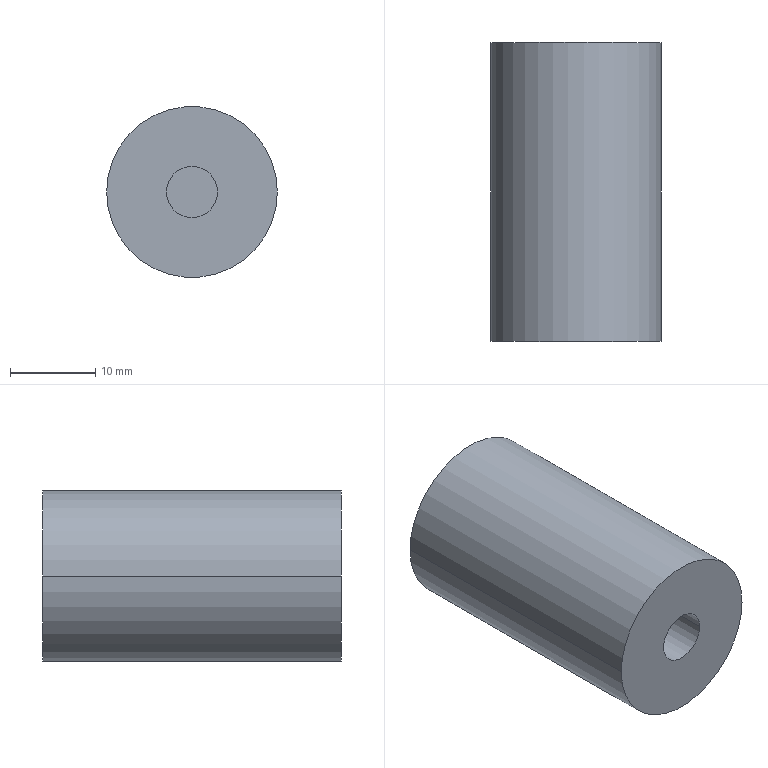Part | STEP file | LIB_58914274 | 1 solid | 10 faces | box 20 x 35 x 20 mm | volume 10543 mm3 | cylinder 6 | plane 4 | commonest cylinder face diameters 6 x4 20 x2
STEP:
#1=CARTESIAN_POINT('',(0.,0.,0.));
#2=DIRECTION('',(0.,0.,1.));
#3=DIRECTION('',(1.,0.,0.));
#4=AXIS2_PLACEMENT_3D('',#1,#2,#3);
#5=CARTESIAN_POINT('',(3.,8.,0.));
#6=VERTEX_POINT('',#5);
#7=CARTESIAN_POINT('',(-3.,8.,0.));
#8=VERTEX_POINT('',#7);
#9=CARTESIAN_POINT('',(0.,8.,0.));
#10=DIRECTION('',(0.,1.,0.));
#11=DIRECTION('',(1.,0.,0.));
#12=AXIS2_PLACEMENT_3D('',#9,#10,#11);
#13=CIRCLE('',#12,3.);
#14=CARTESIAN_POINT('',(0.,8.,0.));
#15=DIRECTION('',(0.,-1.,0.));
#16=DIRECTION('',(-1.,0.,0.));
#17=AXIS2_PLACEMENT_3D('',#14,#15,#16);
#18=PLANE('',#17);
#19=CARTESIAN_POINT('',(-3.,0.));
#20=CARTESIAN_POINT('',(-3.,5.196));
#21=CARTESIAN_POINT('',(1.5,2.598));
#22=CARTESIAN_POINT('',(6.,0.));
#23=CARTESIAN_POINT('',(1.5,-2.598));
#24=CARTESIAN_POINT('',(-3.,-5.196));
#25=CARTESIAN_POINT('',(-3.,0.));
#26=(BOUNDED_CURVE()B_SPLINE_CURVE(2,(#19,#20,#21,#22,#23,#24,#25),.UNSPECIFIED.,.T.,.F.)B_SPLINE_CURVE_WITH_KNOTS((1,2,2,2,2,1),(-2.094,0.,2.094,4.189,6.283,8.378),.UNSPECIFIED.)CURVE()GEOMETRIC_REPRESENTATION_ITEM()RATIONAL_B_SPLINE_CURVE((1.,0.5,1.,0.5,1.,0.5,1.))REPRESENTATION_ITEM(''));
#27=(GEOMETRIC_REPRESENTATION_CONTEXT(2)PARAMETRIC_REPRESENTATION_CONTEXT()REPRESENTATION_CONTEXT('',''));
#28=DEFINITIONAL_REPRESENTATION('',(#26),#27);
#29=PCURVE('',#18,#28);
#30=CARTESIAN_POINT('',(0.,36.75,0.));
#31=DIRECTION('',(0.,-1.,0.));
#32=DIRECTION('',(-1.,0.,0.));
#33=AXIS2_PLACEMENT_3D('',#30,#31,#32);
#34=CYLINDRICAL_SURFACE('',#33,3.);
#35=CARTESIAN_POINT('',(3.142,28.75));
#36=DIRECTION('',(-1.,0.));
#37=VECTOR('',#36,1.);
#38=LINE('',#35,#37);
#39=(GEOMETRIC_REPRESENTATION_CONTEXT(2)PARAMETRIC_REPRESENTATION_CONTEXT()REPRESENTATION_CONTEXT('',''));
#40=DEFINITIONAL_REPRESENTATION('',(#38),#39);
#41=PCURVE('',#34,#40);
#42=SURFACE_CURVE('',#13,(#29,#41),.PCURVE_S1.);
#43=EDGE_CURVE('',#6,#8,#42,.T.);
#44=ORIENTED_EDGE('',*,*,#43,.T.);
#45=CARTESIAN_POINT('',(0.,8.,0.));
#46=DIRECTION('',(0.,-1.,0.));
#47=DIRECTION('',(1.,0.,0.));
#48=AXIS2_PLACEMENT_3D('',#45,#46,#47);
#49=CIRCLE('',#48,3.);
#50=CARTESIAN_POINT('',(0.,0.));
#51=DIRECTION('',(-1.,0.));
#52=AXIS2_PLACEMENT_2D('',#50,#51);
#53=CIRCLE('',#52,3.);
#54=(GEOMETRIC_REPRESENTATION_CONTEXT(2)PARAMETRIC_REPRESENTATION_CONTEXT()REPRESENTATION_CONTEXT('',''));
#55=DEFINITIONAL_REPRESENTATION('',(#53),#54);
#56=PCURVE('',#18,#55);
#57=CARTESIAN_POINT('',(0.,36.75,0.));
#58=DIRECTION('',(0.,-1.,0.));
#59=DIRECTION('',(-1.,0.,0.));
#60=AXIS2_PLACEMENT_3D('',#57,#58,#59);
#61=CYLINDRICAL_SURFACE('',#60,3.);
#62=CARTESIAN_POINT('',(3.142,28.75));
#63=DIRECTION('',(1.,0.));
#64=VECTOR('',#63,1.);
#65=LINE('',#62,#64);
#66=(GEOMETRIC_REPRESENTATION_CONTEXT(2)PARAMETRIC_REPRESENTATION_CONTEXT()REPRESENTATION_CONTEXT('',''));
#67=DEFINITIONAL_REPRESENTATION('',(#65),#66);
#68=PCURVE('',#61,#67);
#69=SURFACE_CURVE('',#49,(#56,#68),.PCURVE_S1.);
#70=EDGE_CURVE('',#6,#8,#69,.T.);
#71=ORIENTED_EDGE('',*,*,#70,.F.);
#72=EDGE_LOOP('',(#44,#71));
#73=FACE_BOUND('',#72,.F.);
#74=ADVANCED_FACE('',(#73),#18,.T.);
#75=CARTESIAN_POINT('',(3.,0.,0.));
#76=VERTEX_POINT('',#75);
#77=CARTESIAN_POINT('',(3.,8.,0.));
#78=DIRECTION('',(0.,-1.,0.));
#79=VECTOR('',#78,1.);
#80=LINE('',#77,#79);
#81=CARTESIAN_POINT('',(3.142,28.75));
#82=DIRECTION('',(0.,1.));
#83=VECTOR('',#82,1.);
#84=LINE('',#81,#83);
#85=(GEOMETRIC_REPRESENTATION_CONTEXT(2)PARAMETRIC_REPRESENTATION_CONTEXT()REPRESENTATION_CONTEXT('',''));
#86=DEFINITIONAL_REPRESENTATION('',(#84),#85);
#87=PCURVE('',#34,#86);
#88=CARTESIAN_POINT('',(3.142,28.75));
#89=DIRECTION('',(0.,1.));
#90=VECTOR('',#89,1.);
#91=LINE('',#88,#90);
#92=(GEOMETRIC_REPRESENTATION_CONTEXT(2)PARAMETRIC_REPRESENTATION_CONTEXT()REPRESENTATION_CONTEXT('',''));
#93=DEFINITIONAL_REPRESENTATION('',(#91),#92);
#94=PCURVE('',#61,#93);
#95=SURFACE_CURVE('',#80,(#87,#94),.PCURVE_S1.);
#96=EDGE_CURVE('',#6,#76,#95,.T.);
#97=ORIENTED_EDGE('',*,*,#96,.T.);
#98=CARTESIAN_POINT('',(-3.,0.,0.));
#99=VERTEX_POINT('',#98);
#100=CARTESIAN_POINT('',(0.,0.,0.));
#101=DIRECTION('',(0.,1.,0.));
#102=DIRECTION('',(1.,0.,0.));
#103=AXIS2_PLACEMENT_3D('',#100,#101,#102);
#104=CIRCLE('',#103,3.);
#105=CARTESIAN_POINT('',(3.142,36.75));
#106=DIRECTION('',(-1.,0.));
#107=VECTOR('',#106,1.);
#108=LINE('',#105,#107);
#109=(GEOMETRIC_REPRESENTATION_CONTEXT(2)PARAMETRIC_REPRESENTATION_CONTEXT()REPRESENTATION_CONTEXT('',''));
#110=DEFINITIONAL_REPRESENTATION('',(#108),#109);
#111=PCURVE('',#34,#110);
#112=CARTESIAN_POINT('',(0.,0.,0.));
#113=DIRECTION('',(0.,-1.,0.));
#114=DIRECTION('',(-1.,0.,0.));
#115=AXIS2_PLACEMENT_3D('',#112,#113,#114);
#116=PLANE('',#115);
#117=CARTESIAN_POINT('',(-3.,0.));
#118=CARTESIAN_POINT('',(-3.,5.196));
#119=CARTESIAN_POINT('',(1.5,2.598));
#120=CARTESIAN_POINT('',(6.,0.));
#121=CARTESIAN_POINT('',(1.5,-2.598));
#122=CARTESIAN_POINT('',(-3.,-5.196));
#123=CARTESIAN_POINT('',(-3.,0.));
#124=(BOUNDED_CURVE()B_SPLINE_CURVE(2,(#117,#118,#119,#120,#121,#122,#123),.UNSPECIFIED.,.T.,.F.)B_SPLINE_CURVE_WITH_KNOTS((1,2,2,2,2,1),(-2.094,0.,2.094,4.189,6.283,8.378),.UNSPECIFIED.)CURVE()GEOMETRIC_REPRESENTATION_ITEM()RATIONAL_B_SPLINE_CURVE((1.,0.5,1.,0.5,1.,0.5,1.))REPRESENTATION_ITEM(''));
#125=(GEOMETRIC_REPRESENTATION_CONTEXT(2)PARAMETRIC_REPRESENTATION_CONTEXT()REPRESENTATION_CONTEXT('',''));
#126=DEFINITIONAL_REPRESENTATION('',(#124),#125);
#127=PCURVE('',#116,#126);
#128=SURFACE_CURVE('',#104,(#111,#127),.PCURVE_S1.);
#129=EDGE_CURVE('',#76,#99,#128,.T.);
#130=ORIENTED_EDGE('',*,*,#129,.T.);
#131=CARTESIAN_POINT('',(-3.,8.,0.));
#132=DIRECTION('',(0.,-1.,0.));
#133=VECTOR('',#132,1.);
#134=LINE('',#131,#133);
#135=CARTESIAN_POINT('',(0.,28.75));
#136=DIRECTION('',(0.,1.));
#137=VECTOR('',#136,1.);
#138=LINE('',#135,#137);
#139=(GEOMETRIC_REPRESENTATION_CONTEXT(2)PARAMETRIC_REPRESENTATION_CONTEXT()REPRESENTATION_CONTEXT('',''));
#140=DEFINITIONAL_REPRESENTATION('',(#138),#139);
#141=PCURVE('',#34,#140);
#142=CARTESIAN_POINT('',(6.283,28.75));
#143=DIRECTION('',(0.,1.));
#144=VECTOR('',#143,1.);
#145=LINE('',#142,#144);
#146=(GEOMETRIC_REPRESENTATION_CONTEXT(2)PARAMETRIC_REPRESENTATION_CONTEXT()REPRESENTATION_CONTEXT('',''));
#147=DEFINITIONAL_REPRESENTATION('',(#145),#146);
#148=PCURVE('',#61,#147);
#149=SURFACE_CURVE('',#134,(#141,#148),.PCURVE_S1.);
#150=EDGE_CURVE('',#8,#99,#149,.T.);
#151=ORIENTED_EDGE('',*,*,#150,.F.);
#152=ORIENTED_EDGE('',*,*,#43,.F.);
#153=EDGE_LOOP('',(#97,#130,#151,#152));
#154=FACE_BOUND('',#153,.F.);
#155=ADVANCED_FACE('',(#154),#34,.F.);
#156=ORIENTED_EDGE('',*,*,#96,.F.);
#157=ORIENTED_EDGE('',*,*,#70,.T.);
#158=ORIENTED_EDGE('',*,*,#150,.T.);
#159=CARTESIAN_POINT('',(0.,0.,0.));
#160=DIRECTION('',(0.,-1.,0.));
#161=DIRECTION('',(1.,0.,0.));
#162=AXIS2_PLACEMENT_3D('',#159,#160,#161);
#163=CIRCLE('',#162,3.);
#164=CARTESIAN_POINT('',(3.142,36.75));
#165=DIRECTION('',(1.,0.));
#166=VECTOR('',#165,1.);
#167=LINE('',#164,#166);
#168=(GEOMETRIC_REPRESENTATION_CONTEXT(2)PARAMETRIC_REPRESENTATION_CONTEXT()REPRESENTATION_CONTEXT('',''));
#169=DEFINITIONAL_REPRESENTATION('',(#167),#168);
#170=PCURVE('',#61,#169);
#171=CARTESIAN_POINT('',(0.,0.));
#172=DIRECTION('',(-1.,0.));
#173=AXIS2_PLACEMENT_2D('',#171,#172);
#174=CIRCLE('',#173,3.);
#175=(GEOMETRIC_REPRESENTATION_CONTEXT(2)PARAMETRIC_REPRESENTATION_CONTEXT()REPRESENTATION_CONTEXT('',''));
#176=DEFINITIONAL_REPRESENTATION('',(#174),#175);
#177=PCURVE('',#116,#176);
#178=SURFACE_CURVE('',#163,(#170,#177),.PCURVE_S1.);
#179=EDGE_CURVE('',#76,#99,#178,.T.);
#180=ORIENTED_EDGE('',*,*,#179,.F.);
#181=EDGE_LOOP('',(#156,#157,#158,#180));
#182=FACE_BOUND('',#181,.F.);
#183=ADVANCED_FACE('',(#182),#61,.F.);
#184=CARTESIAN_POINT('',(10.,0.,0.));
#185=VERTEX_POINT('',#184);
#186=CARTESIAN_POINT('',(-10.,0.,0.));
#187=VERTEX_POINT('',#186);
#188=CARTESIAN_POINT('',(0.,0.,0.));
#189=DIRECTION('',(0.,1.,0.));
#190=DIRECTION('',(1.,0.,0.));
#191=AXIS2_PLACEMENT_3D('',#188,#189,#190);
#192=CIRCLE('',#191,10.);
#193=CARTESIAN_POINT('',(-10.,0.));
#194=CARTESIAN_POINT('',(-10.,17.321));
#195=CARTESIAN_POINT('',(5.,8.66));
#196=CARTESIAN_POINT('',(20.,0.));
#197=CARTESIAN_POINT('',(5.,-8.66));
#198=CARTESIAN_POINT('',(-10.,-17.321));
#199=CARTESIAN_POINT('',(-10.,0.));
#200=(BOUNDED_CURVE()B_SPLINE_CURVE(2,(#193,#194,#195,#196,#197,#198,#199),.UNSPECIFIED.,.T.,.F.)B_SPLINE_CURVE_WITH_KNOTS((1,2,2,2,2,1),(-2.094,0.,2.094,4.189,6.283,8.378),.UNSPECIFIED.)CURVE()GEOMETRIC_REPRESENTATION_ITEM()RATIONAL_B_SPLINE_CURVE((1.,0.5,1.,0.5,1.,0.5,1.))REPRESENTATION_ITEM(''));
#201=(GEOMETRIC_REPRESENTATION_CONTEXT(2)PARAMETRIC_REPRESENTATION_CONTEXT()REPRESENTATION_CONTEXT('',''));
#202=DEFINITIONAL_REPRESENTATION('',(#200),#201);
#203=PCURVE('',#116,#202);
#204=CARTESIAN_POINT('',(0.,36.75,0.));
#205=DIRECTION('',(0.,-1.,0.));
#206=DIRECTION('',(-1.,0.,0.));
#207=AXIS2_PLACEMENT_3D('',#204,#205,#206);
#208=CYLINDRICAL_SURFACE('',#207,10.);
#209=CARTESIAN_POINT('',(3.142,36.75));
#210=DIRECTION('',(-1.,0.));
#211=VECTOR('',#210,1.);
#212=LINE('',#209,#211);
#213=(GEOMETRIC_REPRESENTATION_CONTEXT(2)PARAMETRIC_REPRESENTATION_CONTEXT()REPRESENTATION_CONTEXT('',''));
#214=DEFINITIONAL_REPRESENTATION('',(#212),#213);
#215=PCURVE('',#208,#214);
#216=SURFACE_CURVE('',#192,(#203,#215),.PCURVE_S1.);
#217=EDGE_CURVE('',#185,#187,#216,.T.);
#218=ORIENTED_EDGE('',*,*,#217,.T.);
#219=CARTESIAN_POINT('',(0.,0.,0.));
#220=DIRECTION('',(0.,-1.,0.));
#221=DIRECTION('',(1.,0.,0.));
#222=AXIS2_PLACEMENT_3D('',#219,#220,#221);
#223=CIRCLE('',#222,10.);
#224=CARTESIAN_POINT('',(0.,0.));
#225=DIRECTION('',(-1.,0.));
#226=AXIS2_PLACEMENT_2D('',#224,#225);
#227=CIRCLE('',#226,10.);
#228=(GEOMETRIC_REPRESENTATION_CONTEXT(2)PARAMETRIC_REPRESENTATION_CONTEXT()REPRESENTATION_CONTEXT('',''));
#229=DEFINITIONAL_REPRESENTATION('',(#227),#228);
#230=PCURVE('',#116,#229);
#231=CARTESIAN_POINT('',(0.,36.75,0.));
#232=DIRECTION('',(0.,-1.,0.));
#233=DIRECTION('',(-1.,0.,0.));
#234=AXIS2_PLACEMENT_3D('',#231,#232,#233);
#235=CYLINDRICAL_SURFACE('',#234,10.);
#236=CARTESIAN_POINT('',(3.142,36.75));
#237=DIRECTION('',(1.,0.));
#238=VECTOR('',#237,1.);
#239=LINE('',#236,#238);
#240=(GEOMETRIC_REPRESENTATION_CONTEXT(2)PARAMETRIC_REPRESENTATION_CONTEXT()REPRESENTATION_CONTEXT('',''));
#241=DEFINITIONAL_REPRESENTATION('',(#239),#240);
#242=PCURVE('',#235,#241);
#243=SURFACE_CURVE('',#223,(#230,#242),.PCURVE_S1.);
#244=EDGE_CURVE('',#185,#187,#243,.T.);
#245=ORIENTED_EDGE('',*,*,#244,.F.);
#246=EDGE_LOOP('',(#218,#245));
#247=FACE_BOUND('',#246,.F.);
#248=ORIENTED_EDGE('',*,*,#179,.T.);
#249=ORIENTED_EDGE('',*,*,#129,.F.);
#250=EDGE_LOOP('',(#248,#249));
#251=FACE_BOUND('',#250,.F.);
#252=ADVANCED_FACE('',(#247,#251),#116,.T.);
#253=ORIENTED_EDGE('',*,*,#217,.T.);
#254=CARTESIAN_POINT('',(-10.,35.,0.));
#255=VERTEX_POINT('',#254);
#256=CARTESIAN_POINT('',(-10.,0.,0.));
#257=DIRECTION('',(0.,1.,0.));
#258=VECTOR('',#257,1.);
#259=LINE('',#256,#258);
#260=CARTESIAN_POINT('',(0.,36.75));
#261=DIRECTION('',(0.,-1.));
#262=VECTOR('',#261,1.);
#263=LINE('',#260,#262);
#264=(GEOMETRIC_REPRESENTATION_CONTEXT(2)PARAMETRIC_REPRESENTATION_CONTEXT()REPRESENTATION_CONTEXT('',''));
#265=DEFINITIONAL_REPRESENTATION('',(#263),#264);
#266=PCURVE('',#208,#265);
#267=CARTESIAN_POINT('',(6.283,36.75));
#268=DIRECTION('',(0.,-1.));
#269=VECTOR('',#268,1.);
#270=LINE('',#267,#269);
#271=(GEOMETRIC_REPRESENTATION_CONTEXT(2)PARAMETRIC_REPRESENTATION_CONTEXT()REPRESENTATION_CONTEXT('',''));
#272=DEFINITIONAL_REPRESENTATION('',(#270),#271);
#273=PCURVE('',#235,#272);
#274=SURFACE_CURVE('',#259,(#266,#273),.PCURVE_S1.);
#275=EDGE_CURVE('',#187,#255,#274,.T.);
#276=ORIENTED_EDGE('',*,*,#275,.T.);
#277=CARTESIAN_POINT('',(10.,35.,0.));
#278=VERTEX_POINT('',#277);
#279=CARTESIAN_POINT('',(0.,35.,0.));
#280=DIRECTION('',(0.,1.,0.));
#281=DIRECTION('',(1.,0.,0.));
#282=AXIS2_PLACEMENT_3D('',#279,#280,#281);
#283=CIRCLE('',#282,10.);
#284=CARTESIAN_POINT('',(3.142,1.75));
#285=DIRECTION('',(-1.,0.));
#286=VECTOR('',#285,1.);
#287=LINE('',#284,#286);
#288=(GEOMETRIC_REPRESENTATION_CONTEXT(2)PARAMETRIC_REPRESENTATION_CONTEXT()REPRESENTATION_CONTEXT('',''));
#289=DEFINITIONAL_REPRESENTATION('',(#287),#288);
#290=PCURVE('',#208,#289);
#291=CARTESIAN_POINT('',(0.,35.,0.));
#292=DIRECTION('',(0.,-1.,0.));
#293=DIRECTION('',(-1.,0.,0.));
#294=AXIS2_PLACEMENT_3D('',#291,#292,#293);
#295=PLANE('',#294);
#296=CARTESIAN_POINT('',(-10.,0.));
#297=CARTESIAN_POINT('',(-10.,17.321));
#298=CARTESIAN_POINT('',(5.,8.66));
#299=CARTESIAN_POINT('',(20.,0.));
#300=CARTESIAN_POINT('',(5.,-8.66));
#301=CARTESIAN_POINT('',(-10.,-17.321));
#302=CARTESIAN_POINT('',(-10.,0.));
#303=(BOUNDED_CURVE()B_SPLINE_CURVE(2,(#296,#297,#298,#299,#300,#301,#302),.UNSPECIFIED.,.T.,.F.)B_SPLINE_CURVE_WITH_KNOTS((1,2,2,2,2,1),(-2.094,0.,2.094,4.189,6.283,8.378),.UNSPECIFIED.)CURVE()GEOMETRIC_REPRESENTATION_ITEM()RATIONAL_B_SPLINE_CURVE((1.,0.5,1.,0.5,1.,0.5,1.))REPRESENTATION_ITEM(''));
#304=(GEOMETRIC_REPRESENTATION_CONTEXT(2)PARAMETRIC_REPRESENTATION_CONTEXT()REPRESENTATION_CONTEXT('',''));
#305=DEFINITIONAL_REPRESENTATION('',(#303),#304);
#306=PCURVE('',#295,#305);
#307=SURFACE_CURVE('',#283,(#290,#306),.PCURVE_S1.);
#308=EDGE_CURVE('',#278,#255,#307,.T.);
#309=ORIENTED_EDGE('',*,*,#308,.F.);
#310=CARTESIAN_POINT('',(10.,0.,0.));
#311=DIRECTION('',(0.,1.,0.));
#312=VECTOR('',#311,1.);
#313=LINE('',#310,#312);
#314=CARTESIAN_POINT('',(3.142,36.75));
#315=DIRECTION('',(0.,-1.));
#316=VECTOR('',#315,1.);
#317=LINE('',#314,#316);
#318=(GEOMETRIC_REPRESENTATION_CONTEXT(2)PARAMETRIC_REPRESENTATION_CONTEXT()REPRESENTATION_CONTEXT('',''));
#319=DEFINITIONAL_REPRESENTATION('',(#317),#318);
#320=PCURVE('',#208,#319);
#321=CARTESIAN_POINT('',(3.142,36.75));
#322=DIRECTION('',(0.,-1.));
#323=VECTOR('',#322,1.);
#324=LINE('',#321,#323);
#325=(GEOMETRIC_REPRESENTATION_CONTEXT(2)PARAMETRIC_REPRESENTATION_CONTEXT()REPRESENTATION_CONTEXT('',''));
#326=DEFINITIONAL_REPRESENTATION('',(#324),#325);
#327=PCURVE('',#235,#326);
#328=SURFACE_CURVE('',#313,(#320,#327),.PCURVE_S1.);
#329=EDGE_CURVE('',#185,#278,#328,.T.);
#330=ORIENTED_EDGE('',*,*,#329,.F.);
#331=EDGE_LOOP('',(#253,#276,#309,#330));
#332=FACE_BOUND('',#331,.T.);
#333=ADVANCED_FACE('',(#332),#208,.T.);
#334=CARTESIAN_POINT('',(0.,35.,0.));
#335=DIRECTION('',(0.,-1.,0.));
#336=DIRECTION('',(1.,0.,0.));
#337=AXIS2_PLACEMENT_3D('',#334,#335,#336);
#338=CIRCLE('',#337,10.);
#339=CARTESIAN_POINT('',(3.142,1.75));
#340=DIRECTION('',(1.,0.));
#341=VECTOR('',#340,1.);
#342=LINE('',#339,#341);
#343=(GEOMETRIC_REPRESENTATION_CONTEXT(2)PARAMETRIC_REPRESENTATION_CONTEXT()REPRESENTATION_CONTEXT('',''));
#344=DEFINITIONAL_REPRESENTATION('',(#342),#343);
#345=PCURVE('',#235,#344);
#346=CARTESIAN_POINT('',(0.,0.));
#347=DIRECTION('',(-1.,0.));
#348=AXIS2_PLACEMENT_2D('',#346,#347);
#349=CIRCLE('',#348,10.);
#350=(GEOMETRIC_REPRESENTATION_CONTEXT(2)PARAMETRIC_REPRESENTATION_CONTEXT()REPRESENTATION_CONTEXT('',''));
#351=DEFINITIONAL_REPRESENTATION('',(#349),#350);
#352=PCURVE('',#295,#351);
#353=SURFACE_CURVE('',#338,(#345,#352),.PCURVE_S1.);
#354=EDGE_CURVE('',#278,#255,#353,.T.);
#355=ORIENTED_EDGE('',*,*,#354,.T.);
#356=ORIENTED_EDGE('',*,*,#275,.F.);
#357=ORIENTED_EDGE('',*,*,#244,.F.);
#358=ORIENTED_EDGE('',*,*,#329,.T.);
#359=EDGE_LOOP('',(#355,#356,#357,#358));
#360=FACE_BOUND('',#359,.T.);
#361=ADVANCED_FACE('',(#360),#235,.T.);
#362=ORIENTED_EDGE('',*,*,#354,.T.);
#363=ORIENTED_EDGE('',*,*,#308,.F.);
#364=EDGE_LOOP('',(#362,#363));
#365=FACE_BOUND('',#364,.F.);
#366=CARTESIAN_POINT('',(3.,35.,0.));
#367=VERTEX_POINT('',#366);
#368=CARTESIAN_POINT('',(-3.,35.,0.));
#369=VERTEX_POINT('',#368);
#370=CARTESIAN_POINT('',(0.,35.,0.));
#371=DIRECTION('',(0.,1.,0.));
#372=DIRECTION('',(1.,0.,0.));
#373=AXIS2_PLACEMENT_3D('',#370,#371,#372);
#374=CIRCLE('',#373,3.);
#375=CARTESIAN_POINT('',(-3.,0.));
#376=CARTESIAN_POINT('',(-3.,5.196));
#377=CARTESIAN_POINT('',(1.5,2.598));
#378=CARTESIAN_POINT('',(6.,0.));
#379=CARTESIAN_POINT('',(1.5,-2.598));
#380=CARTESIAN_POINT('',(-3.,-5.196));
#381=CARTESIAN_POINT('',(-3.,0.));
#382=(BOUNDED_CURVE()B_SPLINE_CURVE(2,(#375,#376,#377,#378,#379,#380,#381),.UNSPECIFIED.,.T.,.F.)B_SPLINE_CURVE_WITH_KNOTS((1,2,2,2,2,1),(-2.094,0.,2.094,4.189,6.283,8.378),.UNSPECIFIED.)CURVE()GEOMETRIC_REPRESENTATION_ITEM()RATIONAL_B_SPLINE_CURVE((1.,0.5,1.,0.5,1.,0.5,1.))REPRESENTATION_ITEM(''));
#383=(GEOMETRIC_REPRESENTATION_CONTEXT(2)PARAMETRIC_REPRESENTATION_CONTEXT()REPRESENTATION_CONTEXT('',''));
#384=DEFINITIONAL_REPRESENTATION('',(#382),#383);
#385=PCURVE('',#295,#384);
#386=CARTESIAN_POINT('',(0.,36.75,0.));
#387=DIRECTION('',(0.,-1.,0.));
#388=DIRECTION('',(-1.,0.,0.));
#389=AXIS2_PLACEMENT_3D('',#386,#387,#388);
#390=CYLINDRICAL_SURFACE('',#389,3.);
#391=CARTESIAN_POINT('',(3.142,1.75));
#392=DIRECTION('',(-1.,0.));
#393=VECTOR('',#392,1.);
#394=LINE('',#391,#393);
#395=(GEOMETRIC_REPRESENTATION_CONTEXT(2)PARAMETRIC_REPRESENTATION_CONTEXT()REPRESENTATION_CONTEXT('',''));
#396=DEFINITIONAL_REPRESENTATION('',(#394),#395);
#397=PCURVE('',#390,#396);
#398=SURFACE_CURVE('',#374,(#385,#397),.PCURVE_S1.);
#399=EDGE_CURVE('',#367,#369,#398,.T.);
#400=ORIENTED_EDGE('',*,*,#399,.T.);
#401=CARTESIAN_POINT('',(0.,35.,0.));
#402=DIRECTION('',(0.,-1.,0.));
#403=DIRECTION('',(1.,0.,0.));
#404=AXIS2_PLACEMENT_3D('',#401,#402,#403);
#405=CIRCLE('',#404,3.);
#406=CARTESIAN_POINT('',(0.,0.));
#407=DIRECTION('',(-1.,0.));
#408=AXIS2_PLACEMENT_2D('',#406,#407);
#409=CIRCLE('',#408,3.);
#410=(GEOMETRIC_REPRESENTATION_CONTEXT(2)PARAMETRIC_REPRESENTATION_CONTEXT()REPRESENTATION_CONTEXT('',''));
#411=DEFINITIONAL_REPRESENTATION('',(#409),#410);
#412=PCURVE('',#295,#411);
#413=CARTESIAN_POINT('',(0.,36.75,0.));
#414=DIRECTION('',(0.,-1.,0.));
#415=DIRECTION('',(-1.,0.,0.));
#416=AXIS2_PLACEMENT_3D('',#413,#414,#415);
#417=CYLINDRICAL_SURFACE('',#416,3.);
#418=CARTESIAN_POINT('',(3.142,1.75));
#419=DIRECTION('',(1.,0.));
#420=VECTOR('',#419,1.);
#421=LINE('',#418,#420);
#422=(GEOMETRIC_REPRESENTATION_CONTEXT(2)PARAMETRIC_REPRESENTATION_CONTEXT()REPRESENTATION_CONTEXT('',''));
#423=DEFINITIONAL_REPRESENTATION('',(#421),#422);
#424=PCURVE('',#417,#423);
#425=SURFACE_CURVE('',#405,(#412,#424),.PCURVE_S1.);
#426=EDGE_CURVE('',#367,#369,#425,.T.);
#427=ORIENTED_EDGE('',*,*,#426,.F.);
#428=EDGE_LOOP('',(#400,#427));
#429=FACE_BOUND('',#428,.F.);
#430=ADVANCED_FACE('',(#365,#429),#295,.F.);
#431=CARTESIAN_POINT('',(3.,27.,0.));
#432=VERTEX_POINT('',#431);
#433=CARTESIAN_POINT('',(3.,35.,0.));
#434=DIRECTION('',(0.,-1.,0.));
#435=VECTOR('',#434,1.);
#436=LINE('',#433,#435);
#437=CARTESIAN_POINT('',(3.142,1.75));
#438=DIRECTION('',(0.,1.));
#439=VECTOR('',#438,1.);
#440=LINE('',#437,#439);
#441=(GEOMETRIC_REPRESENTATION_CONTEXT(2)PARAMETRIC_REPRESENTATION_CONTEXT()REPRESENTATION_CONTEXT('',''));
#442=DEFINITIONAL_REPRESENTATION('',(#440),#441);
#443=PCURVE('',#390,#442);
#444=CARTESIAN_POINT('',(3.142,1.75));
#445=DIRECTION('',(0.,1.));
#446=VECTOR('',#445,1.);
#447=LINE('',#444,#446);
#448=(GEOMETRIC_REPRESENTATION_CONTEXT(2)PARAMETRIC_REPRESENTATION_CONTEXT()REPRESENTATION_CONTEXT('',''));
#449=DEFINITIONAL_REPRESENTATION('',(#447),#448);
#450=PCURVE('',#417,#449);
#451=SURFACE_CURVE('',#436,(#443,#450),.PCURVE_S1.);
#452=EDGE_CURVE('',#367,#432,#451,.T.);
#453=ORIENTED_EDGE('',*,*,#452,.T.);
#454=CARTESIAN_POINT('',(-3.,27.,0.));
#455=VERTEX_POINT('',#454);
#456=CARTESIAN_POINT('',(0.,27.,0.));
#457=DIRECTION('',(0.,1.,0.));
#458=DIRECTION('',(1.,0.,0.));
#459=AXIS2_PLACEMENT_3D('',#456,#457,#458);
#460=CIRCLE('',#459,3.);
#461=CARTESIAN_POINT('',(3.142,9.75));
#462=DIRECTION('',(-1.,0.));
#463=VECTOR('',#462,1.);
#464=LINE('',#461,#463);
#465=(GEOMETRIC_REPRESENTATION_CONTEXT(2)PARAMETRIC_REPRESENTATION_CONTEXT()REPRESENTATION_CONTEXT('',''));
#466=DEFINITIONAL_REPRESENTATION('',(#464),#465);
#467=PCURVE('',#390,#466);
#468=CARTESIAN_POINT('',(0.,27.,0.));
#469=DIRECTION('',(0.,-1.,0.));
#470=DIRECTION('',(-1.,0.,0.));
#471=AXIS2_PLACEMENT_3D('',#468,#469,#470);
#472=PLANE('',#471);
#473=CARTESIAN_POINT('',(-3.,0.));
#474=CARTESIAN_POINT('',(-3.,5.196));
#475=CARTESIAN_POINT('',(1.5,2.598));
#476=CARTESIAN_POINT('',(6.,0.));
#477=CARTESIAN_POINT('',(1.5,-2.598));
#478=CARTESIAN_POINT('',(-3.,-5.196));
#479=CARTESIAN_POINT('',(-3.,0.));
#480=(BOUNDED_CURVE()B_SPLINE_CURVE(2,(#473,#474,#475,#476,#477,#478,#479),.UNSPECIFIED.,.T.,.F.)B_SPLINE_CURVE_WITH_KNOTS((1,2,2,2,2,1),(-2.094,0.,2.094,4.189,6.283,8.378),.UNSPECIFIED.)CURVE()GEOMETRIC_REPRESENTATION_ITEM()RATIONAL_B_SPLINE_CURVE((1.,0.5,1.,0.5,1.,0.5,1.))REPRESENTATION_ITEM(''));
#481=(GEOMETRIC_REPRESENTATION_CONTEXT(2)PARAMETRIC_REPRESENTATION_CONTEXT()REPRESENTATION_CONTEXT('',''));
#482=DEFINITIONAL_REPRESENTATION('',(#480),#481);
#483=PCURVE('',#472,#482);
#484=SURFACE_CURVE('',#460,(#467,#483),.PCURVE_S1.);
#485=EDGE_CURVE('',#432,#455,#484,.T.);
#486=ORIENTED_EDGE('',*,*,#485,.T.);
#487=CARTESIAN_POINT('',(-3.,35.,0.));
#488=DIRECTION('',(0.,-1.,0.));
#489=VECTOR('',#488,1.);
#490=LINE('',#487,#489);
#491=CARTESIAN_POINT('',(0.,1.75));
#492=DIRECTION('',(0.,1.));
#493=VECTOR('',#492,1.);
#494=LINE('',#491,#493);
#495=(GEOMETRIC_REPRESENTATION_CONTEXT(2)PARAMETRIC_REPRESENTATION_CONTEXT()REPRESENTATION_CONTEXT('',''));
#496=DEFINITIONAL_REPRESENTATION('',(#494),#495);
#497=PCURVE('',#390,#496);
#498=CARTESIAN_POINT('',(6.283,1.75));
#499=DIRECTION('',(0.,1.));
#500=VECTOR('',#499,1.);
#501=LINE('',#498,#500);
#502=(GEOMETRIC_REPRESENTATION_CONTEXT(2)PARAMETRIC_REPRESENTATION_CONTEXT()REPRESENTATION_CONTEXT('',''));
#503=DEFINITIONAL_REPRESENTATION('',(#501),#502);
#504=PCURVE('',#417,#503);
#505=SURFACE_CURVE('',#490,(#497,#504),.PCURVE_S1.);
#506=EDGE_CURVE('',#369,#455,#505,.T.);
#507=ORIENTED_EDGE('',*,*,#506,.F.);
#508=ORIENTED_EDGE('',*,*,#399,.F.);
#509=EDGE_LOOP('',(#453,#486,#507,#508));
#510=FACE_BOUND('',#509,.F.);
#511=ADVANCED_FACE('',(#510),#390,.F.);
#512=ORIENTED_EDGE('',*,*,#452,.F.);
#513=ORIENTED_EDGE('',*,*,#426,.T.);
#514=ORIENTED_EDGE('',*,*,#506,.T.);
#515=CARTESIAN_POINT('',(0.,27.,0.));
#516=DIRECTION('',(0.,-1.,0.));
#517=DIRECTION('',(1.,0.,0.));
#518=AXIS2_PLACEMENT_3D('',#515,#516,#517);
#519=CIRCLE('',#518,3.);
#520=CARTESIAN_POINT('',(3.142,9.75));
#521=DIRECTION('',(1.,0.));
#522=VECTOR('',#521,1.);
#523=LINE('',#520,#522);
#524=(GEOMETRIC_REPRESENTATION_CONTEXT(2)PARAMETRIC_REPRESENTATION_CONTEXT()REPRESENTATION_CONTEXT('',''));
#525=DEFINITIONAL_REPRESENTATION('',(#523),#524);
#526=PCURVE('',#417,#525);
#527=CARTESIAN_POINT('',(0.,0.));
#528=DIRECTION('',(-1.,0.));
#529=AXIS2_PLACEMENT_2D('',#527,#528);
#530=CIRCLE('',#529,3.);
#531=(GEOMETRIC_REPRESENTATION_CONTEXT(2)PARAMETRIC_REPRESENTATION_CONTEXT()REPRESENTATION_CONTEXT('',''));
#532=DEFINITIONAL_REPRESENTATION('',(#530),#531);
#533=PCURVE('',#472,#532);
#534=SURFACE_CURVE('',#519,(#526,#533),.PCURVE_S1.);
#535=EDGE_CURVE('',#432,#455,#534,.T.);
#536=ORIENTED_EDGE('',*,*,#535,.F.);
#537=EDGE_LOOP('',(#512,#513,#514,#536));
#538=FACE_BOUND('',#537,.F.);
#539=ADVANCED_FACE('',(#538),#417,.F.);
#540=ORIENTED_EDGE('',*,*,#485,.F.);
#541=ORIENTED_EDGE('',*,*,#535,.T.);
#542=EDGE_LOOP('',(#540,#541));
#543=FACE_BOUND('',#542,.F.);
#544=ADVANCED_FACE('',(#543),#472,.F.);
#545=CLOSED_SHELL('',(#74,#155,#183,#252,#333,#361,#430,#511,#539,#544));
#546=MANIFOLD_SOLID_BREP('',#545);
#547=(LENGTH_UNIT()NAMED_UNIT(*)SI_UNIT(.MILLI.,.METRE.));
#548=UNCERTAINTY_MEASURE_WITH_UNIT(LENGTH_MEASURE(0.0000001),#547,'','');
#549=(NAMED_UNIT(*)PLANE_ANGLE_UNIT()SI_UNIT($,.RADIAN.));
#550=(NAMED_UNIT(*)SI_UNIT($,.STERADIAN.)SOLID_ANGLE_UNIT());
#551=(GEOMETRIC_REPRESENTATION_CONTEXT(3)GLOBAL_UNCERTAINTY_ASSIGNED_CONTEXT((#548))GLOBAL_UNIT_ASSIGNED_CONTEXT((#547,#549,#550))REPRESENTATION_CONTEXT('',''));
#552=ADVANCED_BREP_SHAPE_REPRESENTATION('',(#4,#546),#551);